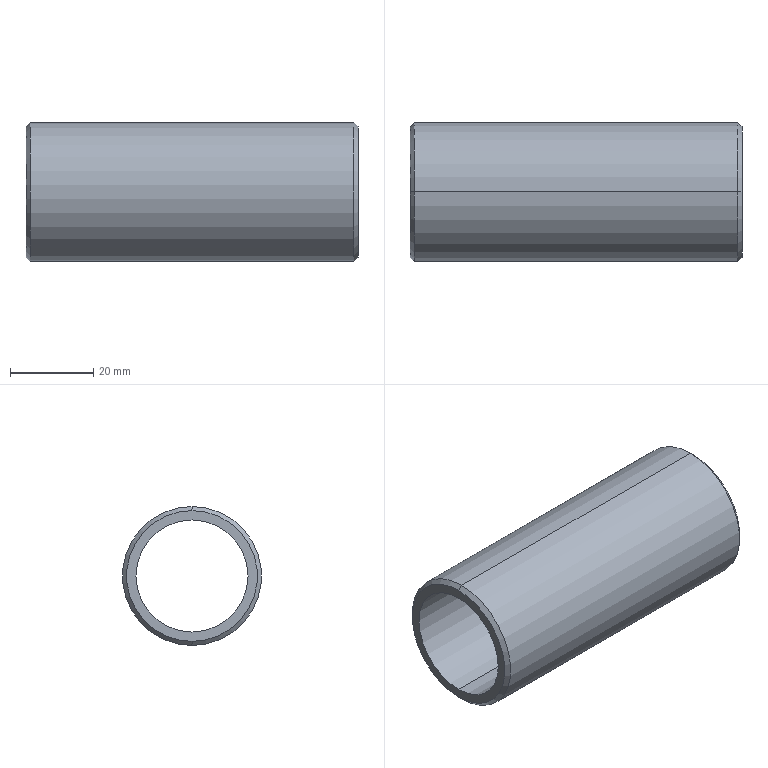Part | SolidWorks | features Chamfer 1, ExtruThin 1 | 1 solid | 10 faces | box 80 x 33.5 x 33.5 mm | volume 24605 mm3 | cone 4 | cylinder 4 | plane 2 | commonest cylinder face diameters 27 x2 33.5 x2
STEP:
#1=CARTESIAN_POINT('',(80.,0.,-15.75));
#2=VERTEX_POINT('',#1);
#3=CARTESIAN_POINT('',(80.,0.,15.75));
#4=VERTEX_POINT('',#3);
#5=CARTESIAN_POINT('',(80.,0.,0.));
#6=DIRECTION('',(1.,0.,0.));
#7=DIRECTION('',(0.,0.,-1.));
#8=AXIS2_PLACEMENT_3D('',#5,#6,#7);
#9=CIRCLE('',#8,15.75);
#10=EDGE_CURVE('',#2,#4,#9,.T.);
#11=ORIENTED_EDGE('',*,*,#10,.F.);
#12=CARTESIAN_POINT('',(79.,0.,-16.75));
#13=VERTEX_POINT('',#12);
#14=CARTESIAN_POINT('',(80.,0.,-15.75));
#15=DIRECTION('',(-0.7071,0.,-0.7071));
#16=VECTOR('',#15,1000.);
#17=LINE('',#14,#16);
#18=EDGE_CURVE('',#2,#13,#17,.T.);
#19=ORIENTED_EDGE('',*,*,#18,.T.);
#20=CARTESIAN_POINT('',(79.,0.,16.75));
#21=VERTEX_POINT('',#20);
#22=CARTESIAN_POINT('',(79.,0.,0.));
#23=DIRECTION('',(-1.,0.,0.));
#24=DIRECTION('',(0.,0.,-1.));
#25=AXIS2_PLACEMENT_3D('',#22,#23,#24);
#26=CIRCLE('',#25,16.75);
#27=EDGE_CURVE('',#21,#13,#26,.T.);
#28=ORIENTED_EDGE('',*,*,#27,.F.);
#29=CARTESIAN_POINT('',(80.,0.,15.75));
#30=DIRECTION('',(-0.7071,0.,0.7071));
#31=VECTOR('',#30,1000.);
#32=LINE('',#29,#31);
#33=EDGE_CURVE('',#4,#21,#32,.T.);
#34=ORIENTED_EDGE('',*,*,#33,.F.);
#35=EDGE_LOOP('',(#11,#19,#28,#34));
#36=FACE_OUTER_BOUND('',#35,.T.);
#37=CARTESIAN_POINT('',(80.,0.,0.));
#38=DIRECTION('',(-1.,0.,0.));
#39=DIRECTION('',(0.,0.,1.));
#40=AXIS2_PLACEMENT_3D('',#37,#38,#39);
#41=CONICAL_SURFACE('',#40,15.75,0.7854);
#42=ADVANCED_FACE('',(#36),#41,.T.);
#43=CARTESIAN_POINT('',(0.,0.,15.75));
#44=VERTEX_POINT('',#43);
#45=CARTESIAN_POINT('',(0.,0.,-15.75));
#46=VERTEX_POINT('',#45);
#47=CARTESIAN_POINT('',(0.,0.,0.));
#48=DIRECTION('',(-1.,0.,0.));
#49=DIRECTION('',(0.,0.,-1.));
#50=AXIS2_PLACEMENT_3D('',#47,#48,#49);
#51=CIRCLE('',#50,15.75);
#52=EDGE_CURVE('',#44,#46,#51,.T.);
#53=ORIENTED_EDGE('',*,*,#52,.F.);
#54=CARTESIAN_POINT('',(1.,0.,16.75));
#55=VERTEX_POINT('',#54);
#56=CARTESIAN_POINT('',(1.,0.,16.75));
#57=DIRECTION('',(0.7071,0.,0.7071));
#58=VECTOR('',#57,1000.);
#59=LINE('',#56,#58);
#60=EDGE_CURVE('',#44,#55,#59,.T.);
#61=ORIENTED_EDGE('',*,*,#60,.T.);
#62=CARTESIAN_POINT('',(1.,0.,-16.75));
#63=VERTEX_POINT('',#62);
#64=CARTESIAN_POINT('',(1.,0.,0.));
#65=DIRECTION('',(1.,0.,0.));
#66=DIRECTION('',(0.,0.,-1.));
#67=AXIS2_PLACEMENT_3D('',#64,#65,#66);
#68=CIRCLE('',#67,16.75);
#69=EDGE_CURVE('',#63,#55,#68,.T.);
#70=ORIENTED_EDGE('',*,*,#69,.F.);
#71=CARTESIAN_POINT('',(1.,0.,-16.75));
#72=DIRECTION('',(0.7071,0.,-0.7071));
#73=VECTOR('',#72,1000.);
#74=LINE('',#71,#73);
#75=EDGE_CURVE('',#46,#63,#74,.T.);
#76=ORIENTED_EDGE('',*,*,#75,.F.);
#77=EDGE_LOOP('',(#53,#61,#70,#76));
#78=FACE_OUTER_BOUND('',#77,.T.);
#79=CARTESIAN_POINT('',(1.,0.,0.));
#80=DIRECTION('',(1.,0.,0.));
#81=DIRECTION('',(0.,0.,-1.));
#82=AXIS2_PLACEMENT_3D('',#79,#80,#81);
#83=CONICAL_SURFACE('',#82,16.75,0.7854);
#84=ADVANCED_FACE('',(#78),#83,.T.);
#85=CARTESIAN_POINT('',(80.,0.,13.5));
#86=VERTEX_POINT('',#85);
#87=CARTESIAN_POINT('',(80.,0.,-13.5));
#88=VERTEX_POINT('',#87);
#89=CARTESIAN_POINT('',(80.,0.,0.));
#90=DIRECTION('',(1.,0.,0.));
#91=DIRECTION('',(0.,0.,-1.));
#92=AXIS2_PLACEMENT_3D('',#89,#90,#91);
#93=CIRCLE('',#92,13.5);
#94=EDGE_CURVE('',#86,#88,#93,.T.);
#95=ORIENTED_EDGE('',*,*,#94,.T.);
#96=CARTESIAN_POINT('',(0.,0.,-13.5));
#97=VERTEX_POINT('',#96);
#98=CARTESIAN_POINT('',(80.,0.,-13.5));
#99=DIRECTION('',(-1.,0.,0.));
#100=VECTOR('',#99,1000.);
#101=LINE('',#98,#100);
#102=EDGE_CURVE('',#88,#97,#101,.T.);
#103=ORIENTED_EDGE('',*,*,#102,.T.);
#104=CARTESIAN_POINT('',(0.,0.,13.5));
#105=VERTEX_POINT('',#104);
#106=CARTESIAN_POINT('',(0.,0.,0.));
#107=DIRECTION('',(1.,0.,0.));
#108=DIRECTION('',(0.,0.,-1.));
#109=AXIS2_PLACEMENT_3D('',#106,#107,#108);
#110=CIRCLE('',#109,13.5);
#111=EDGE_CURVE('',#105,#97,#110,.T.);
#112=ORIENTED_EDGE('',*,*,#111,.F.);
#113=CARTESIAN_POINT('',(80.,0.,13.5));
#114=DIRECTION('',(-1.,0.,0.));
#115=VECTOR('',#114,1000.);
#116=LINE('',#113,#115);
#117=EDGE_CURVE('',#86,#105,#116,.T.);
#118=ORIENTED_EDGE('',*,*,#117,.F.);
#119=EDGE_LOOP('',(#95,#103,#112,#118));
#120=FACE_OUTER_BOUND('',#119,.T.);
#121=CARTESIAN_POINT('',(80.,0.,0.));
#122=DIRECTION('',(-1.,0.,0.));
#123=DIRECTION('',(0.,0.,1.));
#124=AXIS2_PLACEMENT_3D('',#121,#122,#123);
#125=CYLINDRICAL_SURFACE('',#124,13.5);
#126=ADVANCED_FACE('',(#120),#125,.F.);
#127=ORIENTED_EDGE('',*,*,#27,.T.);
#128=CARTESIAN_POINT('',(80.,0.,-16.75));
#129=DIRECTION('',(-1.,0.,0.));
#130=VECTOR('',#129,1000.);
#131=LINE('',#128,#130);
#132=EDGE_CURVE('',#13,#63,#131,.T.);
#133=ORIENTED_EDGE('',*,*,#132,.T.);
#134=ORIENTED_EDGE('',*,*,#69,.T.);
#135=CARTESIAN_POINT('',(80.,0.,16.75));
#136=DIRECTION('',(-1.,0.,0.));
#137=VECTOR('',#136,1000.);
#138=LINE('',#135,#137);
#139=EDGE_CURVE('',#21,#55,#138,.T.);
#140=ORIENTED_EDGE('',*,*,#139,.F.);
#141=EDGE_LOOP('',(#127,#133,#134,#140));
#142=FACE_OUTER_BOUND('',#141,.T.);
#143=CARTESIAN_POINT('',(80.,0.,0.));
#144=DIRECTION('',(-1.,0.,0.));
#145=DIRECTION('',(0.,0.,1.));
#146=AXIS2_PLACEMENT_3D('',#143,#144,#145);
#147=CYLINDRICAL_SURFACE('',#146,16.75);
#148=ADVANCED_FACE('',(#142),#147,.T.);
#149=CARTESIAN_POINT('',(80.,0.,0.));
#150=DIRECTION('',(1.,0.,0.));
#151=DIRECTION('',(0.,0.,-1.));
#152=AXIS2_PLACEMENT_3D('',#149,#150,#151);
#153=CIRCLE('',#152,15.75);
#154=EDGE_CURVE('',#4,#2,#153,.T.);
#155=ORIENTED_EDGE('',*,*,#154,.T.);
#156=ORIENTED_EDGE('',*,*,#10,.T.);
#157=EDGE_LOOP('',(#155,#156));
#158=FACE_OUTER_BOUND('',#157,.T.);
#159=ORIENTED_EDGE('',*,*,#94,.F.);
#160=CARTESIAN_POINT('',(80.,0.,0.));
#161=DIRECTION('',(1.,0.,0.));
#162=DIRECTION('',(0.,0.,-1.));
#163=AXIS2_PLACEMENT_3D('',#160,#161,#162);
#164=CIRCLE('',#163,13.5);
#165=EDGE_CURVE('',#88,#86,#164,.T.);
#166=ORIENTED_EDGE('',*,*,#165,.F.);
#167=EDGE_LOOP('',(#159,#166));
#168=FACE_BOUND('',#167,.T.);
#169=CARTESIAN_POINT('',(80.,0.,0.));
#170=DIRECTION('',(1.,0.,0.));
#171=DIRECTION('',(0.,0.,-1.));
#172=AXIS2_PLACEMENT_3D('',#169,#170,#171);
#173=PLANE('',#172);
#174=ADVANCED_FACE('',(#158,#168),#173,.T.);
#175=CARTESIAN_POINT('',(0.,0.,0.));
#176=DIRECTION('',(-1.,0.,0.));
#177=DIRECTION('',(0.,0.,-1.));
#178=AXIS2_PLACEMENT_3D('',#175,#176,#177);
#179=CIRCLE('',#178,15.75);
#180=EDGE_CURVE('',#46,#44,#179,.T.);
#181=ORIENTED_EDGE('',*,*,#180,.T.);
#182=ORIENTED_EDGE('',*,*,#52,.T.);
#183=EDGE_LOOP('',(#181,#182));
#184=FACE_OUTER_BOUND('',#183,.T.);
#185=ORIENTED_EDGE('',*,*,#111,.T.);
#186=CARTESIAN_POINT('',(0.,0.,0.));
#187=DIRECTION('',(1.,0.,0.));
#188=DIRECTION('',(0.,0.,-1.));
#189=AXIS2_PLACEMENT_3D('',#186,#187,#188);
#190=CIRCLE('',#189,13.5);
#191=EDGE_CURVE('',#97,#105,#190,.T.);
#192=ORIENTED_EDGE('',*,*,#191,.T.);
#193=EDGE_LOOP('',(#185,#192));
#194=FACE_BOUND('',#193,.T.);
#195=CARTESIAN_POINT('',(0.,0.,0.));
#196=DIRECTION('',(1.,0.,0.));
#197=DIRECTION('',(0.,0.,-1.));
#198=AXIS2_PLACEMENT_3D('',#195,#196,#197);
#199=PLANE('',#198);
#200=ADVANCED_FACE('',(#184,#194),#199,.F.);
#201=ORIENTED_EDGE('',*,*,#132,.F.);
#202=CARTESIAN_POINT('',(79.,0.,0.));
#203=DIRECTION('',(-1.,0.,0.));
#204=DIRECTION('',(0.,0.,-1.));
#205=AXIS2_PLACEMENT_3D('',#202,#203,#204);
#206=CIRCLE('',#205,16.75);
#207=EDGE_CURVE('',#13,#21,#206,.T.);
#208=ORIENTED_EDGE('',*,*,#207,.T.);
#209=ORIENTED_EDGE('',*,*,#139,.T.);
#210=CARTESIAN_POINT('',(1.,0.,0.));
#211=DIRECTION('',(1.,0.,0.));
#212=DIRECTION('',(0.,0.,-1.));
#213=AXIS2_PLACEMENT_3D('',#210,#211,#212);
#214=CIRCLE('',#213,16.75);
#215=EDGE_CURVE('',#55,#63,#214,.T.);
#216=ORIENTED_EDGE('',*,*,#215,.T.);
#217=EDGE_LOOP('',(#201,#208,#209,#216));
#218=FACE_OUTER_BOUND('',#217,.T.);
#219=CARTESIAN_POINT('',(80.,0.,0.));
#220=DIRECTION('',(-1.,0.,0.));
#221=DIRECTION('',(0.,0.,1.));
#222=AXIS2_PLACEMENT_3D('',#219,#220,#221);
#223=CYLINDRICAL_SURFACE('',#222,16.75);
#224=ADVANCED_FACE('',(#218),#223,.T.);
#225=ORIENTED_EDGE('',*,*,#102,.F.);
#226=ORIENTED_EDGE('',*,*,#165,.T.);
#227=ORIENTED_EDGE('',*,*,#117,.T.);
#228=ORIENTED_EDGE('',*,*,#191,.F.);
#229=EDGE_LOOP('',(#225,#226,#227,#228));
#230=FACE_OUTER_BOUND('',#229,.T.);
#231=CARTESIAN_POINT('',(80.,0.,0.));
#232=DIRECTION('',(-1.,0.,0.));
#233=DIRECTION('',(0.,0.,1.));
#234=AXIS2_PLACEMENT_3D('',#231,#232,#233);
#235=CYLINDRICAL_SURFACE('',#234,13.5);
#236=ADVANCED_FACE('',(#230),#235,.F.);
#237=ORIENTED_EDGE('',*,*,#60,.F.);
#238=ORIENTED_EDGE('',*,*,#180,.F.);
#239=ORIENTED_EDGE('',*,*,#75,.T.);
#240=ORIENTED_EDGE('',*,*,#215,.F.);
#241=EDGE_LOOP('',(#237,#238,#239,#240));
#242=FACE_OUTER_BOUND('',#241,.T.);
#243=CARTESIAN_POINT('',(1.,0.,0.));
#244=DIRECTION('',(1.,0.,0.));
#245=DIRECTION('',(0.,0.,-1.));
#246=AXIS2_PLACEMENT_3D('',#243,#244,#245);
#247=CONICAL_SURFACE('',#246,16.75,0.7854);
#248=ADVANCED_FACE('',(#242),#247,.T.);
#249=ORIENTED_EDGE('',*,*,#18,.F.);
#250=ORIENTED_EDGE('',*,*,#154,.F.);
#251=ORIENTED_EDGE('',*,*,#33,.T.);
#252=ORIENTED_EDGE('',*,*,#207,.F.);
#253=EDGE_LOOP('',(#249,#250,#251,#252));
#254=FACE_OUTER_BOUND('',#253,.T.);
#255=CARTESIAN_POINT('',(80.,0.,0.));
#256=DIRECTION('',(-1.,0.,0.));
#257=DIRECTION('',(0.,0.,1.));
#258=AXIS2_PLACEMENT_3D('',#255,#256,#257);
#259=CONICAL_SURFACE('',#258,15.75,0.7854);
#260=ADVANCED_FACE('',(#254),#259,.T.);
#261=CLOSED_SHELL('',(#42,#84,#126,#148,#174,#200,#224,#236,#248,#260));
#262=MANIFOLD_SOLID_BREP('',#261);
#263=CARTESIAN_POINT('',(0.,0.,0.));
#264=DIRECTION('',(0.,0.,1.));
#265=DIRECTION('',(1.,0.,0.));
#266=AXIS2_PLACEMENT_3D('',#263,#264,#265);
#267=(LENGTH_UNIT()NAMED_UNIT(*)SI_UNIT(.MILLI.,.METRE.));
#268=UNCERTAINTY_MEASURE_WITH_UNIT(LENGTH_MEASURE(0.00001),#267,'','');
#269=(NAMED_UNIT(*)PLANE_ANGLE_UNIT()SI_UNIT($,.RADIAN.));
#270=(NAMED_UNIT(*)SI_UNIT($,.STERADIAN.)SOLID_ANGLE_UNIT());
#271=(GEOMETRIC_REPRESENTATION_CONTEXT(3)GLOBAL_UNCERTAINTY_ASSIGNED_CONTEXT((#268))GLOBAL_UNIT_ASSIGNED_CONTEXT((#267,#269,#270))REPRESENTATION_CONTEXT('',''));
#272=ADVANCED_BREP_SHAPE_REPRESENTATION('',(#262,#266),#271);